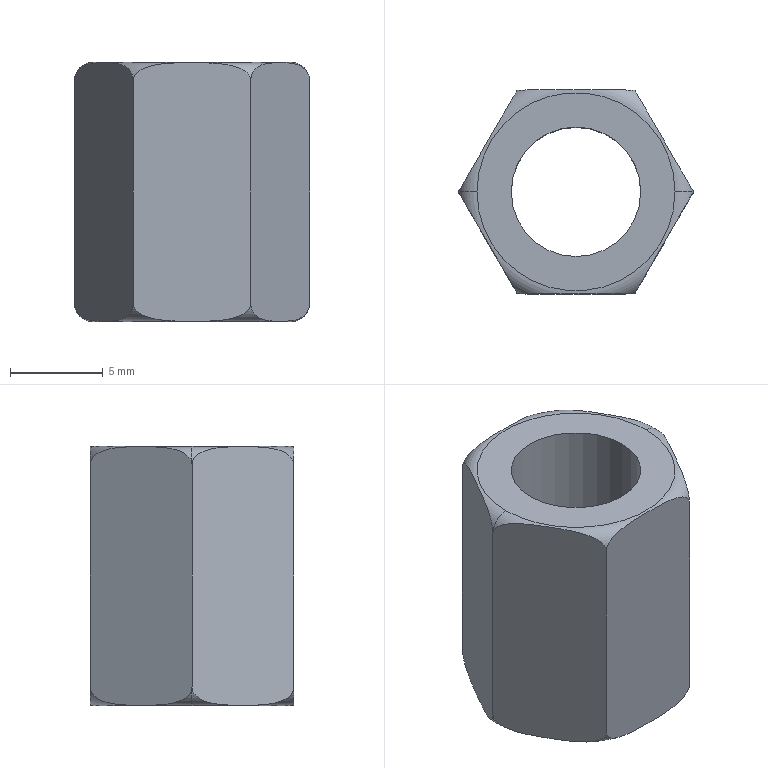Part | STEP file | QA-SKST801 | 1 solid | 14 faces | box 12.702 x 11 x 14 mm | volume 925.966 mm3 | plane 8 | torus 4 | cylinder 2 | commonest cylinder face diameters 7 x2